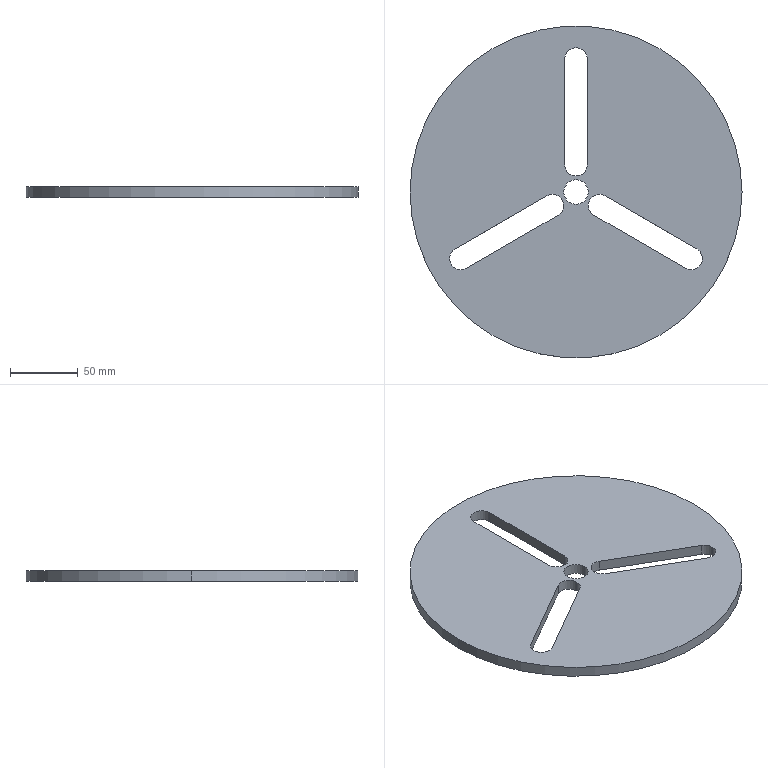Part | STEP file | Tray plate-160 | 1 solid | 20 faces | box 245 x 245 x 8 mm | volume 338994 mm3 | cylinder 12 | plane 8 | commonest cylinder face diameters 16.5 x8 18 x2 245 x2